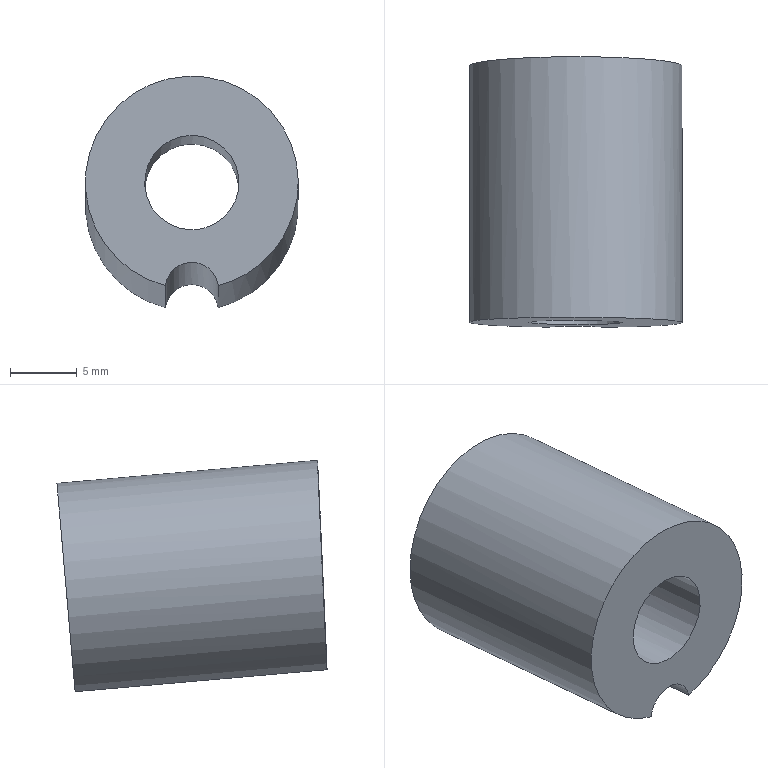Part | NX | features EKSD 16-20-7.100 2 | 1 solid | 7 faces | box 16 x 20.313 x 17.404 mm | volume 2424 mm3 | cylinder 4 | plane 3 | commonest cylinder face diameters 4 x1 7.1 x1 10.6 x1 16 x1
STEP:
#1=CARTESIAN_POINT('',(171.272,-27.467,-40.647));
#2=VERTEX_POINT('',#1);
#3=CARTESIAN_POINT('',(167.304,-27.467,-40.647));
#4=VERTEX_POINT('',#3);
#5=CARTESIAN_POINT('',(169.288,-27.489,-40.896));
#6=DIRECTION('',(0.,-0.9962,0.08716));
#7=DIRECTION('',(0.,0.08716,0.9962));
#8=AXIS2_PLACEMENT_3D('',#5,#6,#7);
#9=CIRCLE('',#8,2.);
#10=EDGE_CURVE('',#2,#4,#9,.T.);
#11=ORIENTED_EDGE('',*,*,#10,.T.);
#12=CARTESIAN_POINT('',(169.288,-26.792,-32.926));
#13=DIRECTION('',(0.,-0.9962,0.08716));
#14=DIRECTION('',(0.,0.08716,0.9962));
#15=AXIS2_PLACEMENT_3D('',#12,#13,#14);
#16=CIRCLE('',#15,8.);
#17=EDGE_CURVE('',#2,#4,#16,.T.);
#18=ORIENTED_EDGE('',*,*,#17,.F.);
#19=EDGE_LOOP('',(#11,#18));
#20=FACE_BOUND('',#19,.T.);
#21=CARTESIAN_POINT('',(169.288,-27.254,-38.206));
#22=VERTEX_POINT('',#21);
#23=CARTESIAN_POINT('',(169.288,-26.792,-32.926));
#24=DIRECTION('',(0.,0.9962,-0.08716));
#25=DIRECTION('',(0.,-0.08716,-0.9962));
#26=AXIS2_PLACEMENT_3D('',#23,#24,#25);
#27=CIRCLE('',#26,5.3);
#28=EDGE_CURVE('',#22,#22,#27,.T.);
#29=ORIENTED_EDGE('',*,*,#28,.F.);
#30=EDGE_LOOP('',(#29));
#31=FACE_BOUND('',#30,.T.);
#32=CARTESIAN_POINT('',(169.288,-26.792,-32.926));
#33=DIRECTION('',(0.,0.9962,-0.08716));
#34=DIRECTION('',(0.,-0.08716,-0.9962));
#35=AXIS2_PLACEMENT_3D('',#32,#33,#34);
#36=PLANE('',#35);
#37=ADVANCED_FACE('',(#20,#31),#36,.T.);
#38=CARTESIAN_POINT('',(167.304,-46.399,-38.991));
#39=VERTEX_POINT('',#38);
#40=CARTESIAN_POINT('',(171.272,-46.407,-38.99));
#41=VERTEX_POINT('',#40);
#42=CARTESIAN_POINT('',(169.288,-46.415,-39.24));
#43=DIRECTION('',(0.001957,0.999,-0.04546));
#44=DIRECTION('',(-0.04675,-0.04532,-0.9979));
#45=AXIS2_PLACEMENT_3D('',#42,#43,#44);
#46=ELLIPSE('',#45,2.002,2.);
#47=EDGE_CURVE('',#39,#41,#46,.T.);
#48=ORIENTED_EDGE('',*,*,#47,.T.);
#49=CARTESIAN_POINT('',(169.288,-46.051,-31.241));
#50=DIRECTION('',(0.001957,0.999,-0.04546));
#51=DIRECTION('',(-0.04675,-0.04532,-0.9979));
#52=AXIS2_PLACEMENT_3D('',#49,#50,#51);
#53=ELLIPSE('',#52,8.007,8.);
#54=EDGE_CURVE('',#39,#41,#53,.T.);
#55=ORIENTED_EDGE('',*,*,#54,.F.);
#56=EDGE_LOOP('',(#48,#55));
#57=FACE_BOUND('',#56,.T.);
#58=CARTESIAN_POINT('',(169.122,-46.212,-34.787));
#59=VERTEX_POINT('',#58);
#60=CARTESIAN_POINT('',(169.288,-46.051,-31.241));
#61=DIRECTION('',(0.001957,0.999,-0.04546));
#62=DIRECTION('',(-0.04675,-0.04532,-0.9979));
#63=AXIS2_PLACEMENT_3D('',#60,#61,#62);
#64=ELLIPSE('',#63,3.553,3.55);
#65=EDGE_CURVE('',#59,#59,#64,.F.);
#66=ORIENTED_EDGE('',*,*,#65,.F.);
#67=EDGE_LOOP('',(#66));
#68=FACE_BOUND('',#67,.T.);
#69=CARTESIAN_POINT('',(128.811,-48.589,-88.763));
#70=DIRECTION('',(0.001957,0.999,-0.04546));
#71=DIRECTION('',(0.06617,0.04523,0.9968));
#72=AXIS2_PLACEMENT_3D('',#69,#70,#71);
#73=PLANE('',#72);
#74=ADVANCED_FACE('',(#57,#68),#73,.F.);
#75=CARTESIAN_POINT('',(167.304,-37.429,-39.775));
#76=DIRECTION('',(0.,0.9962,-0.08716));
#77=VECTOR('',#76,1000.);
#78=LINE('',#75,#77);
#79=EDGE_CURVE('',#39,#4,#78,.T.);
#80=ORIENTED_EDGE('',*,*,#79,.F.);
#81=ORIENTED_EDGE('',*,*,#54,.T.);
#82=CARTESIAN_POINT('',(171.272,-37.429,-39.775));
#83=DIRECTION('',(0.,0.9962,-0.08716));
#84=VECTOR('',#83,1000.);
#85=LINE('',#82,#84);
#86=EDGE_CURVE('',#2,#41,#85,.F.);
#87=ORIENTED_EDGE('',*,*,#86,.F.);
#88=ORIENTED_EDGE('',*,*,#17,.T.);
#89=EDGE_LOOP('',(#80,#81,#87,#88));
#90=FACE_BOUND('',#89,.T.);
#91=CARTESIAN_POINT('',(169.288,-46.716,-31.183));
#92=DIRECTION('',(0.,0.9962,-0.08716));
#93=DIRECTION('',(0.,-0.08716,-0.9962));
#94=AXIS2_PLACEMENT_3D('',#91,#92,#93);
#95=CYLINDRICAL_SURFACE('',#94,8.);
#96=ADVANCED_FACE('',(#90),#95,.T.);
#97=CARTESIAN_POINT('',(169.288,-38.437,-28.344));
#98=VERTEX_POINT('',#97);
#99=CARTESIAN_POINT('',(169.288,-38.746,-31.881));
#100=DIRECTION('',(0.,-0.9962,0.08716));
#101=DIRECTION('',(0.,0.08716,0.9962));
#102=AXIS2_PLACEMENT_3D('',#99,#100,#101);
#103=CIRCLE('',#102,3.55);
#104=EDGE_CURVE('',#98,#98,#103,.F.);
#105=ORIENTED_EDGE('',*,*,#104,.T.);
#106=EDGE_LOOP('',(#105));
#107=FACE_BOUND('',#106,.T.);
#108=ORIENTED_EDGE('',*,*,#65,.T.);
#109=EDGE_LOOP('',(#108));
#110=FACE_BOUND('',#109,.T.);
#111=CARTESIAN_POINT('',(169.288,-47.712,-31.096));
#112=DIRECTION('',(0.,0.9962,-0.08716));
#113=DIRECTION('',(0.,-0.08716,-0.9962));
#114=AXIS2_PLACEMENT_3D('',#111,#112,#113);
#115=CYLINDRICAL_SURFACE('',#114,3.55);
#116=ADVANCED_FACE('',(#107,#110),#115,.F.);
#117=CARTESIAN_POINT('',(169.288,-39.208,-37.16));
#118=VERTEX_POINT('',#117);
#119=CARTESIAN_POINT('',(169.288,-38.746,-31.881));
#120=DIRECTION('',(0.,0.9962,-0.08716));
#121=DIRECTION('',(0.,-0.08716,-0.9962));
#122=AXIS2_PLACEMENT_3D('',#119,#120,#121);
#123=CIRCLE('',#122,5.3);
#124=EDGE_CURVE('',#118,#118,#123,.T.);
#125=ORIENTED_EDGE('',*,*,#124,.T.);
#126=EDGE_LOOP('',(#125));
#127=FACE_BOUND('',#126,.T.);
#128=ORIENTED_EDGE('',*,*,#104,.F.);
#129=EDGE_LOOP('',(#128));
#130=FACE_BOUND('',#129,.T.);
#131=CARTESIAN_POINT('',(169.288,-38.746,-31.881));
#132=DIRECTION('',(0.,-0.9962,0.08716));
#133=DIRECTION('',(0.,0.08716,0.9962));
#134=AXIS2_PLACEMENT_3D('',#131,#132,#133);
#135=PLANE('',#134);
#136=ADVANCED_FACE('',(#127,#130),#135,.F.);
#137=ORIENTED_EDGE('',*,*,#28,.T.);
#138=EDGE_LOOP('',(#137));
#139=FACE_BOUND('',#138,.T.);
#140=ORIENTED_EDGE('',*,*,#124,.F.);
#141=EDGE_LOOP('',(#140));
#142=FACE_BOUND('',#141,.T.);
#143=CARTESIAN_POINT('',(169.288,-38.746,-31.881));
#144=DIRECTION('',(0.,0.9962,-0.08716));
#145=DIRECTION('',(0.,-0.08716,-0.9962));
#146=AXIS2_PLACEMENT_3D('',#143,#144,#145);
#147=CYLINDRICAL_SURFACE('',#146,5.3);
#148=ADVANCED_FACE('',(#139,#142),#147,.F.);
#149=ORIENTED_EDGE('',*,*,#79,.T.);
#150=ORIENTED_EDGE('',*,*,#10,.F.);
#151=ORIENTED_EDGE('',*,*,#86,.T.);
#152=ORIENTED_EDGE('',*,*,#47,.F.);
#153=EDGE_LOOP('',(#149,#150,#151,#152));
#154=FACE_BOUND('',#153,.T.);
#155=CARTESIAN_POINT('',(169.288,-47.413,-39.153));
#156=DIRECTION('',(0.,0.9962,-0.08716));
#157=DIRECTION('',(0.,-0.08716,-0.9962));
#158=AXIS2_PLACEMENT_3D('',#155,#156,#157);
#159=CYLINDRICAL_SURFACE('',#158,2.);
#160=ADVANCED_FACE('',(#154),#159,.F.);
#161=CLOSED_SHELL('',(#37,#74,#96,#116,#136,#148,#160));
#162=MANIFOLD_SOLID_BREP('',#161);
#163=(LENGTH_UNIT()NAMED_UNIT(*)SI_UNIT(.MILLI.,.METRE.));
#164=UNCERTAINTY_MEASURE_WITH_UNIT(LENGTH_MEASURE(0.00001),#163,'','');
#165=(NAMED_UNIT(*)PLANE_ANGLE_UNIT()SI_UNIT($,.RADIAN.));
#166=(NAMED_UNIT(*)SI_UNIT($,.STERADIAN.)SOLID_ANGLE_UNIT());
#167=(GEOMETRIC_REPRESENTATION_CONTEXT(3)GLOBAL_UNCERTAINTY_ASSIGNED_CONTEXT((#164))GLOBAL_UNIT_ASSIGNED_CONTEXT((#163,#165,#166))REPRESENTATION_CONTEXT('',''));
#168=ADVANCED_BREP_SHAPE_REPRESENTATION('',(#162),#167);